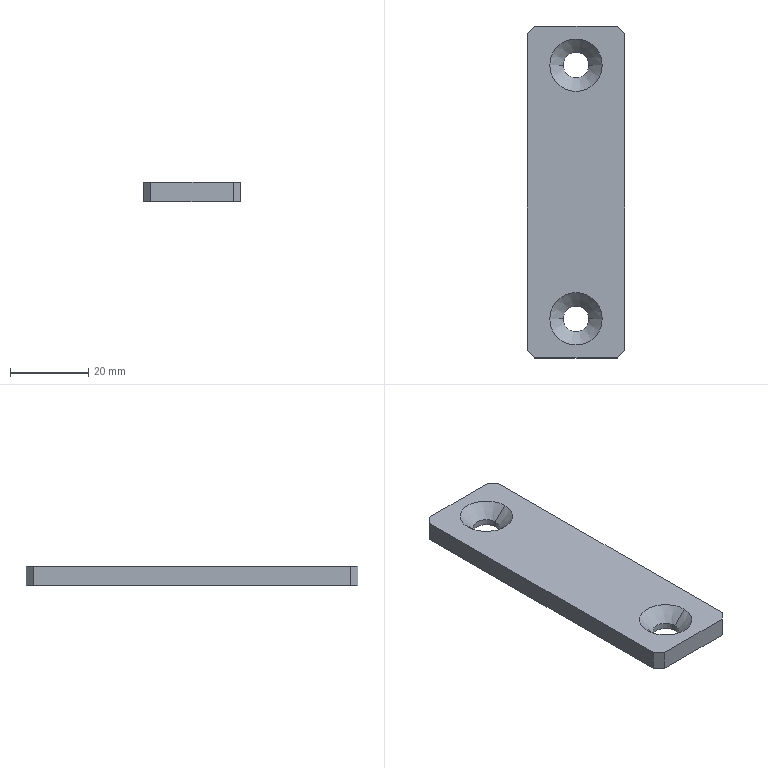Part | SolidWorks | features BaseBody 1 | 1 solid | 18 faces | box 25 x 85 x 5 mm | volume 9917 mm3 | plane 10 | cone 4 | cylinder 4 | commonest cylinder face diameters 6.6 x4
STEP:
#1=CARTESIAN_POINT('',(-798.891,105.,1.58));
#2=VERTEX_POINT('',#1);
#3=CARTESIAN_POINT('',(-792.291,105.,1.58));
#4=VERTEX_POINT('',#3);
#5=CARTESIAN_POINT('',(-795.591,105.,1.58));
#6=DIRECTION('',(0.,0.,1.));
#7=DIRECTION('',(1.,0.,0.));
#8=AXIS2_PLACEMENT_3D('',#5,#6,#7);
#9=CIRCLE('',#8,3.3);
#10=EDGE_CURVE('',#2,#4,#9,.T.);
#11=ORIENTED_EDGE('',*,*,#10,.F.);
#12=CARTESIAN_POINT('',(-802.311,105.,5.));
#13=VERTEX_POINT('',#12);
#14=CARTESIAN_POINT('',(-802.311,105.,5.));
#15=DIRECTION('',(-0.7071,0.,0.7071));
#16=VECTOR('',#15,1000.);
#17=LINE('',#14,#16);
#18=EDGE_CURVE('',#2,#13,#17,.T.);
#19=ORIENTED_EDGE('',*,*,#18,.T.);
#20=CARTESIAN_POINT('',(-788.871,105.,5.));
#21=VERTEX_POINT('',#20);
#22=CARTESIAN_POINT('',(-795.591,105.,5.));
#23=DIRECTION('',(0.,0.,1.));
#24=DIRECTION('',(1.,0.,0.));
#25=AXIS2_PLACEMENT_3D('',#22,#23,#24);
#26=CIRCLE('',#25,6.72);
#27=EDGE_CURVE('',#13,#21,#26,.T.);
#28=ORIENTED_EDGE('',*,*,#27,.T.);
#29=CARTESIAN_POINT('',(-788.871,105.,5.));
#30=DIRECTION('',(0.7071,0.,0.7071));
#31=VECTOR('',#30,1000.);
#32=LINE('',#29,#31);
#33=EDGE_CURVE('',#4,#21,#32,.T.);
#34=ORIENTED_EDGE('',*,*,#33,.F.);
#35=EDGE_LOOP('',(#11,#19,#28,#34));
#36=FACE_OUTER_BOUND('',#35,.T.);
#37=CARTESIAN_POINT('',(-795.591,105.,5.));
#38=DIRECTION('',(0.,0.,1.));
#39=DIRECTION('',(1.,0.,0.));
#40=AXIS2_PLACEMENT_3D('',#37,#38,#39);
#41=CONICAL_SURFACE('',#40,6.72,0.7854);
#42=ADVANCED_FACE('',(#36),#41,.F.);
#43=CARTESIAN_POINT('',(-798.891,105.,0.));
#44=VERTEX_POINT('',#43);
#45=CARTESIAN_POINT('',(-792.291,105.,0.));
#46=VERTEX_POINT('',#45);
#47=CARTESIAN_POINT('',(-795.591,105.,0.));
#48=DIRECTION('',(0.,0.,1.));
#49=DIRECTION('',(1.,0.,0.));
#50=AXIS2_PLACEMENT_3D('',#47,#48,#49);
#51=CIRCLE('',#50,3.3);
#52=EDGE_CURVE('',#44,#46,#51,.T.);
#53=ORIENTED_EDGE('',*,*,#52,.F.);
#54=CARTESIAN_POINT('',(-798.891,105.,5.));
#55=DIRECTION('',(0.,0.,1.));
#56=VECTOR('',#55,1000.);
#57=LINE('',#54,#56);
#58=EDGE_CURVE('',#44,#2,#57,.T.);
#59=ORIENTED_EDGE('',*,*,#58,.T.);
#60=ORIENTED_EDGE('',*,*,#10,.T.);
#61=CARTESIAN_POINT('',(-792.291,105.,5.));
#62=DIRECTION('',(0.,0.,1.));
#63=VECTOR('',#62,1000.);
#64=LINE('',#61,#63);
#65=EDGE_CURVE('',#46,#4,#64,.T.);
#66=ORIENTED_EDGE('',*,*,#65,.F.);
#67=EDGE_LOOP('',(#53,#59,#60,#66));
#68=FACE_OUTER_BOUND('',#67,.T.);
#69=CARTESIAN_POINT('',(-795.591,105.,5.));
#70=DIRECTION('',(0.,0.,1.));
#71=DIRECTION('',(1.,0.,0.));
#72=AXIS2_PLACEMENT_3D('',#69,#70,#71);
#73=CYLINDRICAL_SURFACE('',#72,3.3);
#74=ADVANCED_FACE('',(#68),#73,.F.);
#75=CARTESIAN_POINT('',(-798.891,40.,1.58));
#76=VERTEX_POINT('',#75);
#77=CARTESIAN_POINT('',(-792.291,40.,1.58));
#78=VERTEX_POINT('',#77);
#79=CARTESIAN_POINT('',(-795.591,40.,1.58));
#80=DIRECTION('',(0.,0.,1.));
#81=DIRECTION('',(1.,0.,0.));
#82=AXIS2_PLACEMENT_3D('',#79,#80,#81);
#83=CIRCLE('',#82,3.3);
#84=EDGE_CURVE('',#76,#78,#83,.T.);
#85=ORIENTED_EDGE('',*,*,#84,.F.);
#86=CARTESIAN_POINT('',(-802.311,40.,5.));
#87=VERTEX_POINT('',#86);
#88=CARTESIAN_POINT('',(-802.311,40.,5.));
#89=DIRECTION('',(-0.7071,0.,0.7071));
#90=VECTOR('',#89,1000.);
#91=LINE('',#88,#90);
#92=EDGE_CURVE('',#76,#87,#91,.T.);
#93=ORIENTED_EDGE('',*,*,#92,.T.);
#94=CARTESIAN_POINT('',(-788.871,40.,5.));
#95=VERTEX_POINT('',#94);
#96=CARTESIAN_POINT('',(-795.591,40.,5.));
#97=DIRECTION('',(0.,0.,1.));
#98=DIRECTION('',(1.,0.,0.));
#99=AXIS2_PLACEMENT_3D('',#96,#97,#98);
#100=CIRCLE('',#99,6.72);
#101=EDGE_CURVE('',#87,#95,#100,.T.);
#102=ORIENTED_EDGE('',*,*,#101,.T.);
#103=CARTESIAN_POINT('',(-788.871,40.,5.));
#104=DIRECTION('',(0.7071,0.,0.7071));
#105=VECTOR('',#104,1000.);
#106=LINE('',#103,#105);
#107=EDGE_CURVE('',#78,#95,#106,.T.);
#108=ORIENTED_EDGE('',*,*,#107,.F.);
#109=EDGE_LOOP('',(#85,#93,#102,#108));
#110=FACE_OUTER_BOUND('',#109,.T.);
#111=CARTESIAN_POINT('',(-795.591,40.,5.));
#112=DIRECTION('',(0.,0.,1.));
#113=DIRECTION('',(1.,0.,0.));
#114=AXIS2_PLACEMENT_3D('',#111,#112,#113);
#115=CONICAL_SURFACE('',#114,6.72,0.7854);
#116=ADVANCED_FACE('',(#110),#115,.F.);
#117=CARTESIAN_POINT('',(-798.891,40.,0.));
#118=VERTEX_POINT('',#117);
#119=CARTESIAN_POINT('',(-792.291,40.,0.));
#120=VERTEX_POINT('',#119);
#121=CARTESIAN_POINT('',(-795.591,40.,0.));
#122=DIRECTION('',(0.,0.,1.));
#123=DIRECTION('',(1.,0.,0.));
#124=AXIS2_PLACEMENT_3D('',#121,#122,#123);
#125=CIRCLE('',#124,3.3);
#126=EDGE_CURVE('',#118,#120,#125,.T.);
#127=ORIENTED_EDGE('',*,*,#126,.F.);
#128=CARTESIAN_POINT('',(-798.891,40.,5.));
#129=DIRECTION('',(0.,0.,1.));
#130=VECTOR('',#129,1000.);
#131=LINE('',#128,#130);
#132=EDGE_CURVE('',#118,#76,#131,.T.);
#133=ORIENTED_EDGE('',*,*,#132,.T.);
#134=ORIENTED_EDGE('',*,*,#84,.T.);
#135=CARTESIAN_POINT('',(-792.291,40.,5.));
#136=DIRECTION('',(0.,0.,1.));
#137=VECTOR('',#136,1000.);
#138=LINE('',#135,#137);
#139=EDGE_CURVE('',#120,#78,#138,.T.);
#140=ORIENTED_EDGE('',*,*,#139,.F.);
#141=EDGE_LOOP('',(#127,#133,#134,#140));
#142=FACE_OUTER_BOUND('',#141,.T.);
#143=CARTESIAN_POINT('',(-795.591,40.,5.));
#144=DIRECTION('',(0.,0.,1.));
#145=DIRECTION('',(1.,0.,0.));
#146=AXIS2_PLACEMENT_3D('',#143,#144,#145);
#147=CYLINDRICAL_SURFACE('',#146,3.3);
#148=ADVANCED_FACE('',(#142),#147,.F.);
#149=CARTESIAN_POINT('',(-806.091,115.,5.));
#150=VERTEX_POINT('',#149);
#151=CARTESIAN_POINT('',(-808.091,113.,5.));
#152=VERTEX_POINT('',#151);
#153=CARTESIAN_POINT('',(-460.545,460.545,5.));
#154=DIRECTION('',(-0.7071,-0.7071,0.));
#155=VECTOR('',#154,1000.);
#156=LINE('',#153,#155);
#157=EDGE_CURVE('',#150,#152,#156,.T.);
#158=ORIENTED_EDGE('',*,*,#157,.F.);
#159=CARTESIAN_POINT('',(-806.091,115.,0.));
#160=VERTEX_POINT('',#159);
#161=CARTESIAN_POINT('',(-806.091,115.,5.));
#162=DIRECTION('',(0.,0.,1.));
#163=VECTOR('',#162,1000.);
#164=LINE('',#161,#163);
#165=EDGE_CURVE('',#160,#150,#164,.T.);
#166=ORIENTED_EDGE('',*,*,#165,.F.);
#167=CARTESIAN_POINT('',(-808.091,113.,0.));
#168=VERTEX_POINT('',#167);
#169=CARTESIAN_POINT('',(-808.091,113.,0.));
#170=DIRECTION('',(0.7071,0.7071,0.));
#171=VECTOR('',#170,1000.);
#172=LINE('',#169,#171);
#173=EDGE_CURVE('',#168,#160,#172,.T.);
#174=ORIENTED_EDGE('',*,*,#173,.F.);
#175=CARTESIAN_POINT('',(-808.091,113.,5.));
#176=DIRECTION('',(0.,0.,-1.));
#177=VECTOR('',#176,1000.);
#178=LINE('',#175,#177);
#179=EDGE_CURVE('',#152,#168,#178,.T.);
#180=ORIENTED_EDGE('',*,*,#179,.F.);
#181=EDGE_LOOP('',(#158,#166,#174,#180));
#182=FACE_OUTER_BOUND('',#181,.T.);
#183=CARTESIAN_POINT('',(-808.091,113.,5.));
#184=DIRECTION('',(0.7071,-0.7071,0.));
#185=DIRECTION('',(0.,0.,-1.));
#186=AXIS2_PLACEMENT_3D('',#183,#184,#185);
#187=PLANE('',#186);
#188=ADVANCED_FACE('',(#182),#187,.F.);
#189=CARTESIAN_POINT('',(-783.091,113.,5.));
#190=VERTEX_POINT('',#189);
#191=CARTESIAN_POINT('',(-785.091,115.,5.));
#192=VERTEX_POINT('',#191);
#193=CARTESIAN_POINT('',(-335.045,-335.045,5.));
#194=DIRECTION('',(-0.7071,0.7071,0.));
#195=VECTOR('',#194,1000.);
#196=LINE('',#193,#195);
#197=EDGE_CURVE('',#190,#192,#196,.T.);
#198=ORIENTED_EDGE('',*,*,#197,.F.);
#199=CARTESIAN_POINT('',(-783.091,113.,0.));
#200=VERTEX_POINT('',#199);
#201=CARTESIAN_POINT('',(-783.091,113.,5.));
#202=DIRECTION('',(0.,0.,1.));
#203=VECTOR('',#202,1000.);
#204=LINE('',#201,#203);
#205=EDGE_CURVE('',#200,#190,#204,.T.);
#206=ORIENTED_EDGE('',*,*,#205,.F.);
#207=CARTESIAN_POINT('',(-785.091,115.,0.));
#208=VERTEX_POINT('',#207);
#209=CARTESIAN_POINT('',(-785.091,115.,0.));
#210=DIRECTION('',(0.7071,-0.7071,0.));
#211=VECTOR('',#210,1000.);
#212=LINE('',#209,#211);
#213=EDGE_CURVE('',#208,#200,#212,.T.);
#214=ORIENTED_EDGE('',*,*,#213,.F.);
#215=CARTESIAN_POINT('',(-785.091,115.,5.));
#216=DIRECTION('',(0.,0.,-1.));
#217=VECTOR('',#216,1000.);
#218=LINE('',#215,#217);
#219=EDGE_CURVE('',#192,#208,#218,.T.);
#220=ORIENTED_EDGE('',*,*,#219,.F.);
#221=EDGE_LOOP('',(#198,#206,#214,#220));
#222=FACE_OUTER_BOUND('',#221,.T.);
#223=CARTESIAN_POINT('',(-785.091,115.,5.));
#224=DIRECTION('',(-0.7071,-0.7071,0.));
#225=DIRECTION('',(-0.7071,0.7071,0.));
#226=AXIS2_PLACEMENT_3D('',#223,#224,#225);
#227=PLANE('',#226);
#228=ADVANCED_FACE('',(#222),#227,.F.);
#229=CARTESIAN_POINT('',(-808.091,32.,5.));
#230=VERTEX_POINT('',#229);
#231=CARTESIAN_POINT('',(-806.091,30.,5.));
#232=VERTEX_POINT('',#231);
#233=CARTESIAN_POINT('',(-388.045,-388.045,5.));
#234=DIRECTION('',(0.7071,-0.7071,0.));
#235=VECTOR('',#234,1000.);
#236=LINE('',#233,#235);
#237=EDGE_CURVE('',#230,#232,#236,.T.);
#238=ORIENTED_EDGE('',*,*,#237,.F.);
#239=CARTESIAN_POINT('',(-808.091,32.,0.));
#240=VERTEX_POINT('',#239);
#241=CARTESIAN_POINT('',(-808.091,32.,5.));
#242=DIRECTION('',(0.,0.,1.));
#243=VECTOR('',#242,1000.);
#244=LINE('',#241,#243);
#245=EDGE_CURVE('',#240,#230,#244,.T.);
#246=ORIENTED_EDGE('',*,*,#245,.F.);
#247=CARTESIAN_POINT('',(-806.091,30.,0.));
#248=VERTEX_POINT('',#247);
#249=CARTESIAN_POINT('',(-806.091,30.,0.));
#250=DIRECTION('',(-0.7071,0.7071,0.));
#251=VECTOR('',#250,1000.);
#252=LINE('',#249,#251);
#253=EDGE_CURVE('',#248,#240,#252,.T.);
#254=ORIENTED_EDGE('',*,*,#253,.F.);
#255=CARTESIAN_POINT('',(-806.091,30.,5.));
#256=DIRECTION('',(0.,0.,-1.));
#257=VECTOR('',#256,1000.);
#258=LINE('',#255,#257);
#259=EDGE_CURVE('',#232,#248,#258,.T.);
#260=ORIENTED_EDGE('',*,*,#259,.F.);
#261=EDGE_LOOP('',(#238,#246,#254,#260));
#262=FACE_OUTER_BOUND('',#261,.T.);
#263=CARTESIAN_POINT('',(-806.091,30.,5.));
#264=DIRECTION('',(0.7071,0.7071,0.));
#265=DIRECTION('',(0.,0.,-1.));
#266=AXIS2_PLACEMENT_3D('',#263,#264,#265);
#267=PLANE('',#266);
#268=ADVANCED_FACE('',(#262),#267,.F.);
#269=CARTESIAN_POINT('',(-785.091,30.,5.));
#270=VERTEX_POINT('',#269);
#271=CARTESIAN_POINT('',(-783.091,32.,5.));
#272=VERTEX_POINT('',#271);
#273=CARTESIAN_POINT('',(-407.545,407.545,5.));
#274=DIRECTION('',(0.7071,0.7071,0.));
#275=VECTOR('',#274,1000.);
#276=LINE('',#273,#275);
#277=EDGE_CURVE('',#270,#272,#276,.T.);
#278=ORIENTED_EDGE('',*,*,#277,.F.);
#279=CARTESIAN_POINT('',(-785.091,30.,0.));
#280=VERTEX_POINT('',#279);
#281=CARTESIAN_POINT('',(-785.091,30.,5.));
#282=DIRECTION('',(0.,0.,1.));
#283=VECTOR('',#282,1000.);
#284=LINE('',#281,#283);
#285=EDGE_CURVE('',#280,#270,#284,.T.);
#286=ORIENTED_EDGE('',*,*,#285,.F.);
#287=CARTESIAN_POINT('',(-783.091,32.,0.));
#288=VERTEX_POINT('',#287);
#289=CARTESIAN_POINT('',(-783.091,32.,0.));
#290=DIRECTION('',(-0.7071,-0.7071,0.));
#291=VECTOR('',#290,1000.);
#292=LINE('',#289,#291);
#293=EDGE_CURVE('',#288,#280,#292,.T.);
#294=ORIENTED_EDGE('',*,*,#293,.F.);
#295=CARTESIAN_POINT('',(-783.091,32.,5.));
#296=DIRECTION('',(0.,0.,-1.));
#297=VECTOR('',#296,1000.);
#298=LINE('',#295,#297);
#299=EDGE_CURVE('',#272,#288,#298,.T.);
#300=ORIENTED_EDGE('',*,*,#299,.F.);
#301=EDGE_LOOP('',(#278,#286,#294,#300));
#302=FACE_OUTER_BOUND('',#301,.T.);
#303=CARTESIAN_POINT('',(-783.091,32.,5.));
#304=DIRECTION('',(-0.7071,0.7071,0.));
#305=DIRECTION('',(0.,0.,1.));
#306=AXIS2_PLACEMENT_3D('',#303,#304,#305);
#307=PLANE('',#306);
#308=ADVANCED_FACE('',(#302),#307,.F.);
#309=CARTESIAN_POINT('',(-795.591,40.,0.));
#310=DIRECTION('',(0.,0.,1.));
#311=DIRECTION('',(1.,0.,0.));
#312=AXIS2_PLACEMENT_3D('',#309,#310,#311);
#313=CIRCLE('',#312,3.3);
#314=EDGE_CURVE('',#120,#118,#313,.T.);
#315=ORIENTED_EDGE('',*,*,#314,.T.);
#316=ORIENTED_EDGE('',*,*,#126,.T.);
#317=EDGE_LOOP('',(#315,#316));
#318=FACE_BOUND('',#317,.T.);
#319=CARTESIAN_POINT('',(-795.591,105.,0.));
#320=DIRECTION('',(0.,0.,1.));
#321=DIRECTION('',(1.,0.,0.));
#322=AXIS2_PLACEMENT_3D('',#319,#320,#321);
#323=CIRCLE('',#322,3.3);
#324=EDGE_CURVE('',#46,#44,#323,.T.);
#325=ORIENTED_EDGE('',*,*,#324,.T.);
#326=ORIENTED_EDGE('',*,*,#52,.T.);
#327=EDGE_LOOP('',(#325,#326));
#328=FACE_BOUND('',#327,.T.);
#329=CARTESIAN_POINT('',(-783.091,115.,0.));
#330=DIRECTION('',(0.,1.,0.));
#331=VECTOR('',#330,1000.);
#332=LINE('',#329,#331);
#333=EDGE_CURVE('',#288,#200,#332,.T.);
#334=ORIENTED_EDGE('',*,*,#333,.F.);
#335=ORIENTED_EDGE('',*,*,#293,.T.);
#336=CARTESIAN_POINT('',(-808.091,30.,0.));
#337=DIRECTION('',(1.,0.,0.));
#338=VECTOR('',#337,1000.);
#339=LINE('',#336,#338);
#340=EDGE_CURVE('',#248,#280,#339,.T.);
#341=ORIENTED_EDGE('',*,*,#340,.F.);
#342=ORIENTED_EDGE('',*,*,#253,.T.);
#343=CARTESIAN_POINT('',(-808.091,115.,0.));
#344=DIRECTION('',(0.,-1.,0.));
#345=VECTOR('',#344,1000.);
#346=LINE('',#343,#345);
#347=EDGE_CURVE('',#168,#240,#346,.T.);
#348=ORIENTED_EDGE('',*,*,#347,.F.);
#349=ORIENTED_EDGE('',*,*,#173,.T.);
#350=CARTESIAN_POINT('',(-808.091,115.,0.));
#351=DIRECTION('',(-1.,0.,0.));
#352=VECTOR('',#351,1000.);
#353=LINE('',#350,#352);
#354=EDGE_CURVE('',#208,#160,#353,.T.);
#355=ORIENTED_EDGE('',*,*,#354,.F.);
#356=ORIENTED_EDGE('',*,*,#213,.T.);
#357=EDGE_LOOP('',(#334,#335,#341,#342,#348,#349,#355,#356));
#358=FACE_OUTER_BOUND('',#357,.T.);
#359=CARTESIAN_POINT('',(0.,0.,0.));
#360=DIRECTION('',(0.,0.,1.));
#361=DIRECTION('',(1.,0.,0.));
#362=AXIS2_PLACEMENT_3D('',#359,#360,#361);
#363=PLANE('',#362);
#364=ADVANCED_FACE('',(#318,#328,#358),#363,.F.);
#365=CARTESIAN_POINT('',(-795.591,40.,5.));
#366=DIRECTION('',(0.,0.,1.));
#367=DIRECTION('',(1.,0.,0.));
#368=AXIS2_PLACEMENT_3D('',#365,#366,#367);
#369=CIRCLE('',#368,6.72);
#370=EDGE_CURVE('',#95,#87,#369,.T.);
#371=ORIENTED_EDGE('',*,*,#370,.F.);
#372=ORIENTED_EDGE('',*,*,#101,.F.);
#373=EDGE_LOOP('',(#371,#372));
#374=FACE_BOUND('',#373,.T.);
#375=CARTESIAN_POINT('',(-795.591,105.,5.));
#376=DIRECTION('',(0.,0.,1.));
#377=DIRECTION('',(1.,0.,0.));
#378=AXIS2_PLACEMENT_3D('',#375,#376,#377);
#379=CIRCLE('',#378,6.72);
#380=EDGE_CURVE('',#21,#13,#379,.T.);
#381=ORIENTED_EDGE('',*,*,#380,.F.);
#382=ORIENTED_EDGE('',*,*,#27,.F.);
#383=EDGE_LOOP('',(#381,#382));
#384=FACE_BOUND('',#383,.T.);
#385=CARTESIAN_POINT('',(-808.091,30.,5.));
#386=DIRECTION('',(1.,0.,0.));
#387=VECTOR('',#386,1000.);
#388=LINE('',#385,#387);
#389=EDGE_CURVE('',#232,#270,#388,.T.);
#390=ORIENTED_EDGE('',*,*,#389,.T.);
#391=ORIENTED_EDGE('',*,*,#277,.T.);
#392=CARTESIAN_POINT('',(-783.091,115.,5.));
#393=DIRECTION('',(0.,1.,0.));
#394=VECTOR('',#393,1000.);
#395=LINE('',#392,#394);
#396=EDGE_CURVE('',#272,#190,#395,.T.);
#397=ORIENTED_EDGE('',*,*,#396,.T.);
#398=ORIENTED_EDGE('',*,*,#197,.T.);
#399=CARTESIAN_POINT('',(-808.091,115.,5.));
#400=DIRECTION('',(-1.,0.,0.));
#401=VECTOR('',#400,1000.);
#402=LINE('',#399,#401);
#403=EDGE_CURVE('',#192,#150,#402,.T.);
#404=ORIENTED_EDGE('',*,*,#403,.T.);
#405=ORIENTED_EDGE('',*,*,#157,.T.);
#406=CARTESIAN_POINT('',(-808.091,115.,5.));
#407=DIRECTION('',(0.,-1.,0.));
#408=VECTOR('',#407,1000.);
#409=LINE('',#406,#408);
#410=EDGE_CURVE('',#152,#230,#409,.T.);
#411=ORIENTED_EDGE('',*,*,#410,.T.);
#412=ORIENTED_EDGE('',*,*,#237,.T.);
#413=EDGE_LOOP('',(#390,#391,#397,#398,#404,#405,#411,#412));
#414=FACE_OUTER_BOUND('',#413,.T.);
#415=CARTESIAN_POINT('',(0.,0.,5.));
#416=DIRECTION('',(0.,0.,1.));
#417=DIRECTION('',(1.,0.,0.));
#418=AXIS2_PLACEMENT_3D('',#415,#416,#417);
#419=PLANE('',#418);
#420=ADVANCED_FACE('',(#374,#384,#414),#419,.T.);
#421=ORIENTED_EDGE('',*,*,#403,.F.);
#422=ORIENTED_EDGE('',*,*,#219,.T.);
#423=ORIENTED_EDGE('',*,*,#354,.T.);
#424=ORIENTED_EDGE('',*,*,#165,.T.);
#425=EDGE_LOOP('',(#421,#422,#423,#424));
#426=FACE_OUTER_BOUND('',#425,.T.);
#427=CARTESIAN_POINT('',(-808.091,115.,5.));
#428=DIRECTION('',(0.,-1.,0.));
#429=DIRECTION('',(0.,0.,-1.));
#430=AXIS2_PLACEMENT_3D('',#427,#428,#429);
#431=PLANE('',#430);
#432=ADVANCED_FACE('',(#426),#431,.F.);
#433=ORIENTED_EDGE('',*,*,#396,.F.);
#434=ORIENTED_EDGE('',*,*,#299,.T.);
#435=ORIENTED_EDGE('',*,*,#333,.T.);
#436=ORIENTED_EDGE('',*,*,#205,.T.);
#437=EDGE_LOOP('',(#433,#434,#435,#436));
#438=FACE_OUTER_BOUND('',#437,.T.);
#439=CARTESIAN_POINT('',(-783.091,115.,5.));
#440=DIRECTION('',(-1.,0.,0.));
#441=DIRECTION('',(0.,0.,1.));
#442=AXIS2_PLACEMENT_3D('',#439,#440,#441);
#443=PLANE('',#442);
#444=ADVANCED_FACE('',(#438),#443,.F.);
#445=ORIENTED_EDGE('',*,*,#340,.T.);
#446=ORIENTED_EDGE('',*,*,#285,.T.);
#447=ORIENTED_EDGE('',*,*,#389,.F.);
#448=ORIENTED_EDGE('',*,*,#259,.T.);
#449=EDGE_LOOP('',(#445,#446,#447,#448));
#450=FACE_OUTER_BOUND('',#449,.T.);
#451=CARTESIAN_POINT('',(-808.091,30.,5.));
#452=DIRECTION('',(0.,1.,0.));
#453=DIRECTION('',(1.,0.,0.));
#454=AXIS2_PLACEMENT_3D('',#451,#452,#453);
#455=PLANE('',#454);
#456=ADVANCED_FACE('',(#450),#455,.F.);
#457=ORIENTED_EDGE('',*,*,#347,.T.);
#458=ORIENTED_EDGE('',*,*,#245,.T.);
#459=ORIENTED_EDGE('',*,*,#410,.F.);
#460=ORIENTED_EDGE('',*,*,#179,.T.);
#461=EDGE_LOOP('',(#457,#458,#459,#460));
#462=FACE_OUTER_BOUND('',#461,.T.);
#463=CARTESIAN_POINT('',(-808.091,115.,5.));
#464=DIRECTION('',(1.,0.,0.));
#465=DIRECTION('',(0.,1.,0.));
#466=AXIS2_PLACEMENT_3D('',#463,#464,#465);
#467=PLANE('',#466);
#468=ADVANCED_FACE('',(#462),#467,.F.);
#469=ORIENTED_EDGE('',*,*,#132,.F.);
#470=ORIENTED_EDGE('',*,*,#314,.F.);
#471=ORIENTED_EDGE('',*,*,#139,.T.);
#472=CARTESIAN_POINT('',(-795.591,40.,1.58));
#473=DIRECTION('',(0.,0.,1.));
#474=DIRECTION('',(1.,0.,0.));
#475=AXIS2_PLACEMENT_3D('',#472,#473,#474);
#476=CIRCLE('',#475,3.3);
#477=EDGE_CURVE('',#78,#76,#476,.T.);
#478=ORIENTED_EDGE('',*,*,#477,.T.);
#479=EDGE_LOOP('',(#469,#470,#471,#478));
#480=FACE_OUTER_BOUND('',#479,.T.);
#481=CARTESIAN_POINT('',(-795.591,40.,5.));
#482=DIRECTION('',(0.,0.,1.));
#483=DIRECTION('',(1.,0.,0.));
#484=AXIS2_PLACEMENT_3D('',#481,#482,#483);
#485=CYLINDRICAL_SURFACE('',#484,3.3);
#486=ADVANCED_FACE('',(#480),#485,.F.);
#487=ORIENTED_EDGE('',*,*,#92,.F.);
#488=ORIENTED_EDGE('',*,*,#477,.F.);
#489=ORIENTED_EDGE('',*,*,#107,.T.);
#490=ORIENTED_EDGE('',*,*,#370,.T.);
#491=EDGE_LOOP('',(#487,#488,#489,#490));
#492=FACE_OUTER_BOUND('',#491,.T.);
#493=CARTESIAN_POINT('',(-795.591,40.,5.));
#494=DIRECTION('',(0.,0.,1.));
#495=DIRECTION('',(1.,0.,0.));
#496=AXIS2_PLACEMENT_3D('',#493,#494,#495);
#497=CONICAL_SURFACE('',#496,6.72,0.7854);
#498=ADVANCED_FACE('',(#492),#497,.F.);
#499=ORIENTED_EDGE('',*,*,#58,.F.);
#500=ORIENTED_EDGE('',*,*,#324,.F.);
#501=ORIENTED_EDGE('',*,*,#65,.T.);
#502=CARTESIAN_POINT('',(-795.591,105.,1.58));
#503=DIRECTION('',(0.,0.,1.));
#504=DIRECTION('',(1.,0.,0.));
#505=AXIS2_PLACEMENT_3D('',#502,#503,#504);
#506=CIRCLE('',#505,3.3);
#507=EDGE_CURVE('',#4,#2,#506,.T.);
#508=ORIENTED_EDGE('',*,*,#507,.T.);
#509=EDGE_LOOP('',(#499,#500,#501,#508));
#510=FACE_OUTER_BOUND('',#509,.T.);
#511=CARTESIAN_POINT('',(-795.591,105.,5.));
#512=DIRECTION('',(0.,0.,1.));
#513=DIRECTION('',(1.,0.,0.));
#514=AXIS2_PLACEMENT_3D('',#511,#512,#513);
#515=CYLINDRICAL_SURFACE('',#514,3.3);
#516=ADVANCED_FACE('',(#510),#515,.F.);
#517=ORIENTED_EDGE('',*,*,#18,.F.);
#518=ORIENTED_EDGE('',*,*,#507,.F.);
#519=ORIENTED_EDGE('',*,*,#33,.T.);
#520=ORIENTED_EDGE('',*,*,#380,.T.);
#521=EDGE_LOOP('',(#517,#518,#519,#520));
#522=FACE_OUTER_BOUND('',#521,.T.);
#523=CARTESIAN_POINT('',(-795.591,105.,5.));
#524=DIRECTION('',(0.,0.,1.));
#525=DIRECTION('',(1.,0.,0.));
#526=AXIS2_PLACEMENT_3D('',#523,#524,#525);
#527=CONICAL_SURFACE('',#526,6.72,0.7854);
#528=ADVANCED_FACE('',(#522),#527,.F.);
#529=CLOSED_SHELL('',(#42,#74,#116,#148,#188,#228,#268,#308,#364,#420,#432,#444,#456,#468,#486,#498,#516,#528));
#530=MANIFOLD_SOLID_BREP('',#529);
#531=CARTESIAN_POINT('',(0.,0.,0.));
#532=DIRECTION('',(0.,0.,1.));
#533=DIRECTION('',(1.,0.,0.));
#534=AXIS2_PLACEMENT_3D('',#531,#532,#533);
#535=(LENGTH_UNIT()NAMED_UNIT(*)SI_UNIT(.MILLI.,.METRE.));
#536=UNCERTAINTY_MEASURE_WITH_UNIT(LENGTH_MEASURE(0.00001),#535,'','');
#537=(NAMED_UNIT(*)PLANE_ANGLE_UNIT()SI_UNIT($,.RADIAN.));
#538=(NAMED_UNIT(*)SI_UNIT($,.STERADIAN.)SOLID_ANGLE_UNIT());
#539=(GEOMETRIC_REPRESENTATION_CONTEXT(3)GLOBAL_UNCERTAINTY_ASSIGNED_CONTEXT((#536))GLOBAL_UNIT_ASSIGNED_CONTEXT((#535,#537,#538))REPRESENTATION_CONTEXT('',''));
#540=ADVANCED_BREP_SHAPE_REPRESENTATION('',(#530,#534),#539);